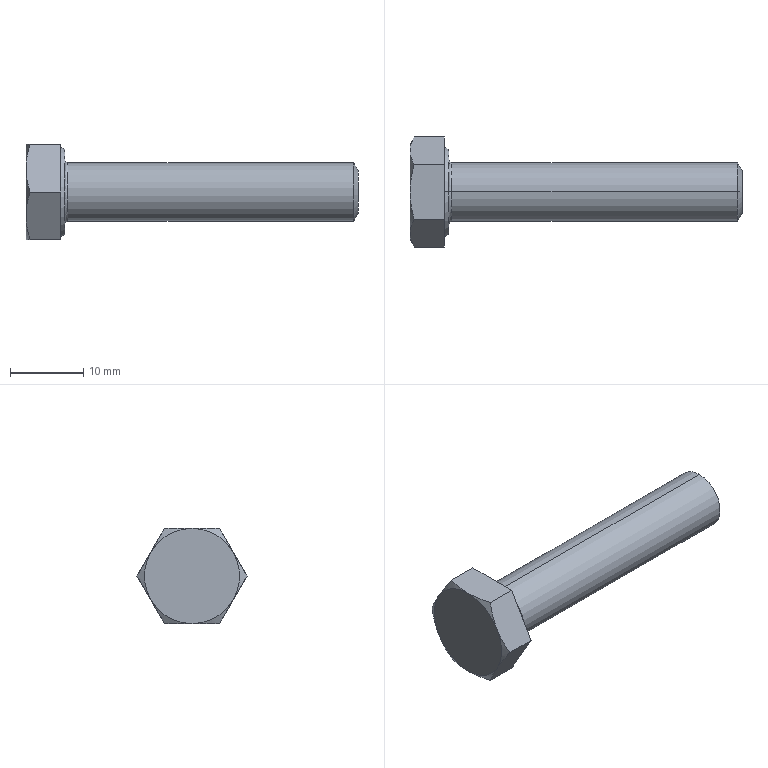Part | SolidWorks | features BaseBody 1, RefAxis 1 | 1 solid | 24 faces | box 45.3 x 15.011 x 13 mm | volume 2757 mm3 | cone 10 | plane 10 | spline 2 | cylinder 2 | commonest cylinder face diameters 8 x2
STEP:
#1=CARTESIAN_POINT('',(5.3,0.,4.4));
#2=VERTEX_POINT('',#1);
#3=CARTESIAN_POINT('',(5.3,0.,-4.4));
#4=VERTEX_POINT('',#3);
#5=CARTESIAN_POINT('',(5.3,0.,4.4));
#6=CARTESIAN_POINT('',(5.3,0.2797,4.4));
#7=CARTESIAN_POINT('',(5.3,0.6919,4.361));
#8=CARTESIAN_POINT('',(5.3,1.16,4.249));
#9=CARTESIAN_POINT('',(5.3,1.391,4.176));
#10=CARTESIAN_POINT('',(5.3,1.489,4.141));
#11=CARTESIAN_POINT('',(5.3,1.554,4.116));
#12=CARTESIAN_POINT('',(5.3,1.585,4.105));
#13=CARTESIAN_POINT('',(5.3,1.758,4.036));
#14=CARTESIAN_POINT('',(5.3,1.96,3.944));
#15=CARTESIAN_POINT('',(5.3,2.154,3.837));
#16=CARTESIAN_POINT('',(5.3,2.282,3.763));
#17=CARTESIAN_POINT('',(5.3,2.344,3.724));
#18=CARTESIAN_POINT('',(5.3,2.662,3.517));
#19=CARTESIAN_POINT('',(5.3,2.897,3.326));
#20=CARTESIAN_POINT('',(5.3,3.219,3.004));
#21=CARTESIAN_POINT('',(5.3,3.37,2.836));
#22=CARTESIAN_POINT('',(5.3,3.509,2.656));
#23=CARTESIAN_POINT('',(5.3,3.598,2.534));
#24=CARTESIAN_POINT('',(5.3,3.642,2.47));
#25=CARTESIAN_POINT('',(5.3,3.764,2.283));
#26=CARTESIAN_POINT('',(5.3,3.876,2.092));
#27=CARTESIAN_POINT('',(5.3,3.989,1.859));
#28=CARTESIAN_POINT('',(5.3,4.042,1.74));
#29=CARTESIAN_POINT('',(5.3,4.063,1.689));
#30=CARTESIAN_POINT('',(5.3,4.077,1.654));
#31=CARTESIAN_POINT('',(5.3,4.085,1.636));
#32=CARTESIAN_POINT('',(5.3,4.297,1.1));
#33=CARTESIAN_POINT('',(5.3,4.4,0.5592));
#34=CARTESIAN_POINT('',(5.3,4.4,-0.2796));
#35=CARTESIAN_POINT('',(5.3,4.361,-0.6917));
#36=CARTESIAN_POINT('',(5.3,4.249,-1.16));
#37=CARTESIAN_POINT('',(5.3,4.176,-1.391));
#38=CARTESIAN_POINT('',(5.3,4.141,-1.489));
#39=CARTESIAN_POINT('',(5.3,4.116,-1.554));
#40=CARTESIAN_POINT('',(5.3,4.105,-1.585));
#41=CARTESIAN_POINT('',(5.3,4.036,-1.758));
#42=CARTESIAN_POINT('',(5.3,3.944,-1.96));
#43=CARTESIAN_POINT('',(5.3,3.837,-2.154));
#44=CARTESIAN_POINT('',(5.3,3.763,-2.282));
#45=CARTESIAN_POINT('',(5.3,3.724,-2.344));
#46=CARTESIAN_POINT('',(5.3,3.517,-2.662));
#47=CARTESIAN_POINT('',(5.3,3.326,-2.897));
#48=CARTESIAN_POINT('',(5.3,3.004,-3.219));
#49=CARTESIAN_POINT('',(5.3,2.836,-3.37));
#50=CARTESIAN_POINT('',(5.3,2.656,-3.509));
#51=CARTESIAN_POINT('',(5.3,2.534,-3.598));
#52=CARTESIAN_POINT('',(5.3,2.47,-3.642));
#53=CARTESIAN_POINT('',(5.3,2.283,-3.764));
#54=CARTESIAN_POINT('',(5.3,2.092,-3.876));
#55=CARTESIAN_POINT('',(5.3,1.859,-3.989));
#56=CARTESIAN_POINT('',(5.3,1.74,-4.042));
#57=CARTESIAN_POINT('',(5.3,1.689,-4.063));
#58=CARTESIAN_POINT('',(5.3,1.654,-4.077));
#59=CARTESIAN_POINT('',(5.3,1.636,-4.085));
#60=CARTESIAN_POINT('',(5.3,1.1,-4.297));
#61=CARTESIAN_POINT('',(5.3,0.5597,-4.4));
#62=CARTESIAN_POINT('',(5.3,0.,-4.4));
#63=B_SPLINE_CURVE_WITH_KNOTS('',3,(#5,#6,#7,#8,#9,#10,#11,#12,#13,#14,#15,#16,#17,#18,#19,#20,#21,#22,#23,#24,#25,#26,#27,#28,#29,#30,#31,#32,#33,#34,#35,#36,#37,#38,#39,#40,#41,#42,#43,#44,#45,#46,#47,#48,#49,#50,#51,#52,#53,#54,#55,#56,#57,#58,#59,#60,#61,#62),.UNSPECIFIED.,.F.,.F.,(4,1,1,1,2,2,1,2,2,2,1,2,2,1,1,1,2,2,2,1,1,1,2,2,1,2,2,2,1,2,2,1,1,1,2,2,4),(0.,0.0625,0.09375,0.1094,0.1172,0.125,0.1562,0.1719,0.1875,0.25,0.2812,0.2969,0.3125,0.3437,0.3594,0.3672,0.3711,0.375,0.5,0.5625,0.5937,0.6094,0.6172,0.625,0.6562,0.6719,0.6875,0.75,0.7812,0.7969,0.8125,0.8437,0.8594,0.8672,0.8711,0.875,1.),.UNSPECIFIED.);
#64=EDGE_CURVE('',#2,#4,#63,.T.);
#65=ORIENTED_EDGE('',*,*,#64,.F.);
#66=CARTESIAN_POINT('',(5.7,0.,4.));
#67=VERTEX_POINT('',#66);
#68=CARTESIAN_POINT('',(5.7,0.,4.4));
#69=DIRECTION('',(0.,-1.,0.));
#70=DIRECTION('',(0.,0.,1.));
#71=AXIS2_PLACEMENT_3D('',#68,#69,#70);
#72=CIRCLE('',#71,0.4);
#73=EDGE_CURVE('',#2,#67,#72,.T.);
#74=ORIENTED_EDGE('',*,*,#73,.T.);
#75=CARTESIAN_POINT('',(5.7,0.,-4.));
#76=VERTEX_POINT('',#75);
#77=CARTESIAN_POINT('',(5.7,0.,0.));
#78=DIRECTION('',(1.,0.,0.));
#79=DIRECTION('',(0.,0.,1.));
#80=AXIS2_PLACEMENT_3D('',#77,#78,#79);
#81=CIRCLE('',#80,4.);
#82=EDGE_CURVE('',#76,#67,#81,.T.);
#83=ORIENTED_EDGE('',*,*,#82,.F.);
#84=CARTESIAN_POINT('',(5.7,0.,-4.4));
#85=DIRECTION('',(0.,1.,0.));
#86=DIRECTION('',(0.,0.,-1.));
#87=AXIS2_PLACEMENT_3D('',#84,#85,#86);
#88=CIRCLE('',#87,0.4);
#89=EDGE_CURVE('',#4,#76,#88,.T.);
#90=ORIENTED_EDGE('',*,*,#89,.F.);
#91=EDGE_LOOP('',(#65,#74,#83,#90));
#92=FACE_OUTER_BOUND('',#91,.T.);
#93=CARTESIAN_POINT('',(5.3,0.,-4.4));
#94=CARTESIAN_POINT('',(5.3,8.8,-4.4));
#95=CARTESIAN_POINT('',(5.3,8.8,4.4));
#96=CARTESIAN_POINT('',(5.3,0.,4.4));
#97=CARTESIAN_POINT('',(5.3,0.,-4.166));
#98=CARTESIAN_POINT('',(5.3,8.331,-4.166));
#99=CARTESIAN_POINT('',(5.3,8.331,4.166));
#100=CARTESIAN_POINT('',(5.3,0.,4.166));
#101=CARTESIAN_POINT('',(5.466,0.,-4.));
#102=CARTESIAN_POINT('',(5.466,8.,-4.));
#103=CARTESIAN_POINT('',(5.466,8.,4.));
#104=CARTESIAN_POINT('',(5.466,0.,4.));
#105=CARTESIAN_POINT('',(5.7,0.,-4.));
#106=CARTESIAN_POINT('',(5.7,8.,-4.));
#107=CARTESIAN_POINT('',(5.7,8.,4.));
#108=CARTESIAN_POINT('',(5.7,0.,4.));
#109=(BOUNDED_SURFACE()B_SPLINE_SURFACE(3,3,((#93,#94,#95,#96),(#97,#98,#99,#100),(#101,#102,#103,#104),(#105,#106,#107,#108)),.UNSPECIFIED.,.F.,.F.,.T.)B_SPLINE_SURFACE_WITH_KNOTS((4,4),(4,4),(0.,1.),(0.,1.),.UNSPECIFIED.)GEOMETRIC_REPRESENTATION_ITEM()RATIONAL_B_SPLINE_SURFACE(((1.,0.3333,0.3333,1.),(0.8047,0.2682,0.2682,0.8047),(0.8047,0.2682,0.2682,0.8047),(1.,0.3333,0.3333,1.)))REPRESENTATION_ITEM('')SURFACE());
#110=ADVANCED_FACE('',(#92),#109,.F.);
#111=CARTESIAN_POINT('',(44.675,0.,4.));
#112=VERTEX_POINT('',#111);
#113=CARTESIAN_POINT('',(44.675,0.,-4.));
#114=VERTEX_POINT('',#113);
#115=CARTESIAN_POINT('',(44.675,0.,0.));
#116=DIRECTION('',(-1.,0.,0.));
#117=DIRECTION('',(0.,0.,1.));
#118=AXIS2_PLACEMENT_3D('',#115,#116,#117);
#119=CIRCLE('',#118,4.);
#120=EDGE_CURVE('',#112,#114,#119,.T.);
#121=ORIENTED_EDGE('',*,*,#120,.T.);
#122=CARTESIAN_POINT('',(0.,0.,-4.));
#123=DIRECTION('',(-1.,0.,0.));
#124=VECTOR('',#123,1000.);
#125=LINE('',#122,#124);
#126=EDGE_CURVE('',#114,#76,#125,.T.);
#127=ORIENTED_EDGE('',*,*,#126,.T.);
#128=ORIENTED_EDGE('',*,*,#82,.T.);
#129=CARTESIAN_POINT('',(0.,0.,4.));
#130=DIRECTION('',(-1.,0.,0.));
#131=VECTOR('',#130,1000.);
#132=LINE('',#129,#131);
#133=EDGE_CURVE('',#112,#67,#132,.T.);
#134=ORIENTED_EDGE('',*,*,#133,.F.);
#135=EDGE_LOOP('',(#121,#127,#128,#134));
#136=FACE_OUTER_BOUND('',#135,.T.);
#137=CARTESIAN_POINT('',(0.,0.,0.));
#138=DIRECTION('',(-1.,0.,0.));
#139=DIRECTION('',(0.,0.,1.));
#140=AXIS2_PLACEMENT_3D('',#137,#138,#139);
#141=CYLINDRICAL_SURFACE('',#140,4.);
#142=ADVANCED_FACE('',(#136),#141,.T.);
#143=CARTESIAN_POINT('',(45.3,0.,2.917));
#144=VERTEX_POINT('',#143);
#145=CARTESIAN_POINT('',(45.3,0.,-2.917));
#146=VERTEX_POINT('',#145);
#147=CARTESIAN_POINT('',(45.3,0.,0.));
#148=DIRECTION('',(-1.,0.,0.));
#149=DIRECTION('',(0.,0.,1.));
#150=AXIS2_PLACEMENT_3D('',#147,#148,#149);
#151=CIRCLE('',#150,2.917);
#152=EDGE_CURVE('',#144,#146,#151,.T.);
#153=ORIENTED_EDGE('',*,*,#152,.T.);
#154=CARTESIAN_POINT('',(44.675,0.,-4.));
#155=DIRECTION('',(-0.5,0.,-0.866));
#156=VECTOR('',#155,1000.);
#157=LINE('',#154,#156);
#158=EDGE_CURVE('',#146,#114,#157,.T.);
#159=ORIENTED_EDGE('',*,*,#158,.T.);
#160=ORIENTED_EDGE('',*,*,#120,.F.);
#161=CARTESIAN_POINT('',(44.675,0.,4.));
#162=DIRECTION('',(-0.5,0.,0.866));
#163=VECTOR('',#162,1000.);
#164=LINE('',#161,#163);
#165=EDGE_CURVE('',#144,#112,#164,.T.);
#166=ORIENTED_EDGE('',*,*,#165,.F.);
#167=EDGE_LOOP('',(#153,#159,#160,#166));
#168=FACE_OUTER_BOUND('',#167,.T.);
#169=CARTESIAN_POINT('',(44.675,0.,0.));
#170=DIRECTION('',(-1.,0.,0.));
#171=DIRECTION('',(0.,0.,1.));
#172=AXIS2_PLACEMENT_3D('',#169,#170,#171);
#173=CONICAL_SURFACE('',#172,4.,1.047);
#174=ADVANCED_FACE('',(#168),#173,.T.);
#175=CARTESIAN_POINT('',(5.3,0.,-5.815));
#176=VERTEX_POINT('',#175);
#177=CARTESIAN_POINT('',(5.3,0.,5.815));
#178=VERTEX_POINT('',#177);
#179=CARTESIAN_POINT('',(5.3,0.,0.));
#180=DIRECTION('',(1.,0.,0.));
#181=DIRECTION('',(0.,0.,1.));
#182=AXIS2_PLACEMENT_3D('',#179,#180,#181);
#183=CIRCLE('',#182,5.815);
#184=EDGE_CURVE('',#176,#178,#183,.T.);
#185=ORIENTED_EDGE('',*,*,#184,.F.);
#186=CARTESIAN_POINT('',(4.7,0.,-6.161));
#187=VERTEX_POINT('',#186);
#188=CARTESIAN_POINT('',(4.7,0.,-6.161));
#189=DIRECTION('',(-0.866,0.,-0.5));
#190=VECTOR('',#189,1000.);
#191=LINE('',#188,#190);
#192=EDGE_CURVE('',#176,#187,#191,.T.);
#193=ORIENTED_EDGE('',*,*,#192,.T.);
#194=CARTESIAN_POINT('',(4.7,0.,6.161));
#195=VERTEX_POINT('',#194);
#196=CARTESIAN_POINT('',(4.7,0.,0.));
#197=DIRECTION('',(1.,0.,0.));
#198=DIRECTION('',(0.,0.,1.));
#199=AXIS2_PLACEMENT_3D('',#196,#197,#198);
#200=CIRCLE('',#199,6.161);
#201=EDGE_CURVE('',#187,#195,#200,.T.);
#202=ORIENTED_EDGE('',*,*,#201,.T.);
#203=CARTESIAN_POINT('',(4.7,0.,6.161));
#204=DIRECTION('',(-0.866,0.,0.5));
#205=VECTOR('',#204,1000.);
#206=LINE('',#203,#205);
#207=EDGE_CURVE('',#178,#195,#206,.T.);
#208=ORIENTED_EDGE('',*,*,#207,.F.);
#209=EDGE_LOOP('',(#185,#193,#202,#208));
#210=FACE_OUTER_BOUND('',#209,.T.);
#211=CARTESIAN_POINT('',(4.7,0.,0.));
#212=DIRECTION('',(-1.,0.,0.));
#213=DIRECTION('',(0.,0.,1.));
#214=AXIS2_PLACEMENT_3D('',#211,#212,#213);
#215=CONICAL_SURFACE('',#214,6.161,0.5236);
#216=ADVANCED_FACE('',(#210),#215,.T.);
#217=ORIENTED_EDGE('',*,*,#126,.F.);
#218=CARTESIAN_POINT('',(44.675,0.,0.));
#219=DIRECTION('',(-1.,0.,0.));
#220=DIRECTION('',(0.,0.,1.));
#221=AXIS2_PLACEMENT_3D('',#218,#219,#220);
#222=CIRCLE('',#221,4.);
#223=EDGE_CURVE('',#114,#112,#222,.T.);
#224=ORIENTED_EDGE('',*,*,#223,.T.);
#225=ORIENTED_EDGE('',*,*,#133,.T.);
#226=CARTESIAN_POINT('',(5.7,0.,0.));
#227=DIRECTION('',(1.,0.,0.));
#228=DIRECTION('',(0.,0.,1.));
#229=AXIS2_PLACEMENT_3D('',#226,#227,#228);
#230=CIRCLE('',#229,4.);
#231=EDGE_CURVE('',#67,#76,#230,.T.);
#232=ORIENTED_EDGE('',*,*,#231,.T.);
#233=EDGE_LOOP('',(#217,#224,#225,#232));
#234=FACE_OUTER_BOUND('',#233,.T.);
#235=CARTESIAN_POINT('',(0.,0.,0.));
#236=DIRECTION('',(-1.,0.,0.));
#237=DIRECTION('',(0.,0.,1.));
#238=AXIS2_PLACEMENT_3D('',#235,#236,#237);
#239=CYLINDRICAL_SURFACE('',#238,4.);
#240=ADVANCED_FACE('',(#234),#239,.T.);
#241=ORIENTED_EDGE('',*,*,#73,.F.);
#242=CARTESIAN_POINT('',(5.3,0.,-4.4));
#243=CARTESIAN_POINT('',(5.3,-0.2797,-4.4));
#244=CARTESIAN_POINT('',(5.3,-0.6919,-4.361));
#245=CARTESIAN_POINT('',(5.3,-1.16,-4.249));
#246=CARTESIAN_POINT('',(5.3,-1.391,-4.176));
#247=CARTESIAN_POINT('',(5.3,-1.489,-4.141));
#248=CARTESIAN_POINT('',(5.3,-1.554,-4.116));
#249=CARTESIAN_POINT('',(5.3,-1.585,-4.105));
#250=CARTESIAN_POINT('',(5.3,-1.758,-4.036));
#251=CARTESIAN_POINT('',(5.3,-1.96,-3.944));
#252=CARTESIAN_POINT('',(5.3,-2.154,-3.837));
#253=CARTESIAN_POINT('',(5.3,-2.282,-3.763));
#254=CARTESIAN_POINT('',(5.3,-2.344,-3.724));
#255=CARTESIAN_POINT('',(5.3,-2.662,-3.517));
#256=CARTESIAN_POINT('',(5.3,-2.897,-3.326));
#257=CARTESIAN_POINT('',(5.3,-3.219,-3.004));
#258=CARTESIAN_POINT('',(5.3,-3.37,-2.836));
#259=CARTESIAN_POINT('',(5.3,-3.509,-2.656));
#260=CARTESIAN_POINT('',(5.3,-3.598,-2.534));
#261=CARTESIAN_POINT('',(5.3,-3.642,-2.47));
#262=CARTESIAN_POINT('',(5.3,-3.764,-2.283));
#263=CARTESIAN_POINT('',(5.3,-3.876,-2.092));
#264=CARTESIAN_POINT('',(5.3,-3.989,-1.859));
#265=CARTESIAN_POINT('',(5.3,-4.042,-1.74));
#266=CARTESIAN_POINT('',(5.3,-4.063,-1.689));
#267=CARTESIAN_POINT('',(5.3,-4.077,-1.654));
#268=CARTESIAN_POINT('',(5.3,-4.085,-1.636));
#269=CARTESIAN_POINT('',(5.3,-4.297,-1.1));
#270=CARTESIAN_POINT('',(5.3,-4.4,-0.5592));
#271=CARTESIAN_POINT('',(5.3,-4.4,0.2796));
#272=CARTESIAN_POINT('',(5.3,-4.361,0.6917));
#273=CARTESIAN_POINT('',(5.3,-4.249,1.16));
#274=CARTESIAN_POINT('',(5.3,-4.176,1.391));
#275=CARTESIAN_POINT('',(5.3,-4.141,1.489));
#276=CARTESIAN_POINT('',(5.3,-4.116,1.554));
#277=CARTESIAN_POINT('',(5.3,-4.105,1.585));
#278=CARTESIAN_POINT('',(5.3,-4.036,1.758));
#279=CARTESIAN_POINT('',(5.3,-3.944,1.96));
#280=CARTESIAN_POINT('',(5.3,-3.837,2.154));
#281=CARTESIAN_POINT('',(5.3,-3.763,2.282));
#282=CARTESIAN_POINT('',(5.3,-3.724,2.344));
#283=CARTESIAN_POINT('',(5.3,-3.517,2.662));
#284=CARTESIAN_POINT('',(5.3,-3.326,2.897));
#285=CARTESIAN_POINT('',(5.3,-3.004,3.219));
#286=CARTESIAN_POINT('',(5.3,-2.836,3.37));
#287=CARTESIAN_POINT('',(5.3,-2.656,3.509));
#288=CARTESIAN_POINT('',(5.3,-2.534,3.598));
#289=CARTESIAN_POINT('',(5.3,-2.47,3.642));
#290=CARTESIAN_POINT('',(5.3,-2.283,3.764));
#291=CARTESIAN_POINT('',(5.3,-2.092,3.876));
#292=CARTESIAN_POINT('',(5.3,-1.859,3.989));
#293=CARTESIAN_POINT('',(5.3,-1.74,4.042));
#294=CARTESIAN_POINT('',(5.3,-1.689,4.063));
#295=CARTESIAN_POINT('',(5.3,-1.654,4.077));
#296=CARTESIAN_POINT('',(5.3,-1.636,4.085));
#297=CARTESIAN_POINT('',(5.3,-1.1,4.297));
#298=CARTESIAN_POINT('',(5.3,-0.5597,4.4));
#299=CARTESIAN_POINT('',(5.3,0.,4.4));
#300=B_SPLINE_CURVE_WITH_KNOTS('',3,(#242,#243,#244,#245,#246,#247,#248,#249,#250,#251,#252,#253,#254,#255,#256,#257,#258,#259,#260,#261,#262,#263,#264,#265,#266,#267,#268,#269,#270,#271,#272,#273,#274,#275,#276,#277,#278,#279,#280,#281,#282,#283,#284,#285,#286,#287,#288,#289,#290,#291,#292,#293,#294,#295,#296,#297,#298,#299),.UNSPECIFIED.,.F.,.F.,(4,1,1,1,2,2,1,2,2,2,1,2,2,1,1,1,2,2,2,1,1,1,2,2,1,2,2,2,1,2,2,1,1,1,2,2,4),(0.,0.0625,0.09375,0.1094,0.1172,0.125,0.1563,0.1719,0.1875,0.25,0.2813,0.2969,0.3125,0.3438,0.3594,0.3672,0.3711,0.375,0.5,0.5625,0.5938,0.6094,0.6172,0.625,0.6563,0.6719,0.6875,0.75,0.7813,0.7969,0.8125,0.8438,0.8594,0.8672,0.8711,0.875,1.),.UNSPECIFIED.);
#301=EDGE_CURVE('',#4,#2,#300,.T.);
#302=ORIENTED_EDGE('',*,*,#301,.F.);
#303=ORIENTED_EDGE('',*,*,#89,.T.);
#304=ORIENTED_EDGE('',*,*,#231,.F.);
#305=EDGE_LOOP('',(#241,#302,#303,#304));
#306=FACE_OUTER_BOUND('',#305,.T.);
#307=CARTESIAN_POINT('',(5.3,0.,4.4));
#308=CARTESIAN_POINT('',(5.3,-8.8,4.4));
#309=CARTESIAN_POINT('',(5.3,-8.8,-4.4));
#310=CARTESIAN_POINT('',(5.3,0.,-4.4));
#311=CARTESIAN_POINT('',(5.3,0.,4.166));
#312=CARTESIAN_POINT('',(5.3,-8.331,4.166));
#313=CARTESIAN_POINT('',(5.3,-8.331,-4.166));
#314=CARTESIAN_POINT('',(5.3,0.,-4.166));
#315=CARTESIAN_POINT('',(5.466,0.,4.));
#316=CARTESIAN_POINT('',(5.466,-8.,4.));
#317=CARTESIAN_POINT('',(5.466,-8.,-4.));
#318=CARTESIAN_POINT('',(5.466,0.,-4.));
#319=CARTESIAN_POINT('',(5.7,0.,4.));
#320=CARTESIAN_POINT('',(5.7,-8.,4.));
#321=CARTESIAN_POINT('',(5.7,-8.,-4.));
#322=CARTESIAN_POINT('',(5.7,0.,-4.));
#323=(BOUNDED_SURFACE()B_SPLINE_SURFACE(3,3,((#307,#308,#309,#310),(#311,#312,#313,#314),(#315,#316,#317,#318),(#319,#320,#321,#322)),.UNSPECIFIED.,.F.,.F.,.T.)B_SPLINE_SURFACE_WITH_KNOTS((4,4),(4,4),(0.,1.),(0.,1.),.UNSPECIFIED.)GEOMETRIC_REPRESENTATION_ITEM()RATIONAL_B_SPLINE_SURFACE(((1.,0.3333,0.3333,1.),(0.8047,0.2682,0.2682,0.8047),(0.8047,0.2682,0.2682,0.8047),(1.,0.3333,0.3333,1.)))REPRESENTATION_ITEM('')SURFACE());
#324=ADVANCED_FACE('',(#306),#323,.F.);
#325=ORIENTED_EDGE('',*,*,#158,.F.);
#326=CARTESIAN_POINT('',(45.3,0.,0.));
#327=DIRECTION('',(-1.,0.,0.));
#328=DIRECTION('',(0.,0.,1.));
#329=AXIS2_PLACEMENT_3D('',#326,#327,#328);
#330=CIRCLE('',#329,2.917);
#331=EDGE_CURVE('',#146,#144,#330,.T.);
#332=ORIENTED_EDGE('',*,*,#331,.T.);
#333=ORIENTED_EDGE('',*,*,#165,.T.);
#334=ORIENTED_EDGE('',*,*,#223,.F.);
#335=EDGE_LOOP('',(#325,#332,#333,#334));
#336=FACE_OUTER_BOUND('',#335,.T.);
#337=CARTESIAN_POINT('',(44.675,0.,0.));
#338=DIRECTION('',(-1.,0.,0.));
#339=DIRECTION('',(0.,0.,1.));
#340=AXIS2_PLACEMENT_3D('',#337,#338,#339);
#341=CONICAL_SURFACE('',#340,4.,1.047);
#342=ADVANCED_FACE('',(#336),#341,.T.);
#343=CARTESIAN_POINT('',(5.3,0.,0.));
#344=DIRECTION('',(1.,0.,0.));
#345=DIRECTION('',(0.,0.,1.));
#346=AXIS2_PLACEMENT_3D('',#343,#344,#345);
#347=CIRCLE('',#346,5.815);
#348=EDGE_CURVE('',#178,#176,#347,.T.);
#349=ORIENTED_EDGE('',*,*,#348,.T.);
#350=ORIENTED_EDGE('',*,*,#184,.T.);
#351=EDGE_LOOP('',(#349,#350));
#352=FACE_OUTER_BOUND('',#351,.T.);
#353=ORIENTED_EDGE('',*,*,#301,.T.);
#354=ORIENTED_EDGE('',*,*,#64,.T.);
#355=EDGE_LOOP('',(#353,#354));
#356=FACE_BOUND('',#355,.T.);
#357=CARTESIAN_POINT('',(5.3,0.,-13.));
#358=DIRECTION('',(1.,0.,0.));
#359=DIRECTION('',(0.,0.,-1.));
#360=AXIS2_PLACEMENT_3D('',#357,#358,#359);
#361=PLANE('',#360);
#362=ADVANCED_FACE('',(#352,#356),#361,.T.);
#363=ORIENTED_EDGE('',*,*,#152,.F.);
#364=ORIENTED_EDGE('',*,*,#331,.F.);
#365=EDGE_LOOP('',(#363,#364));
#366=FACE_OUTER_BOUND('',#365,.T.);
#367=CARTESIAN_POINT('',(45.3,0.,0.));
#368=DIRECTION('',(-1.,0.,0.));
#369=DIRECTION('',(0.,0.,1.));
#370=AXIS2_PLACEMENT_3D('',#367,#368,#369);
#371=PLANE('',#370);
#372=ADVANCED_FACE('',(#366),#371,.F.);
#373=ORIENTED_EDGE('',*,*,#192,.F.);
#374=ORIENTED_EDGE('',*,*,#348,.F.);
#375=ORIENTED_EDGE('',*,*,#207,.T.);
#376=CARTESIAN_POINT('',(4.7,0.,0.));
#377=DIRECTION('',(1.,0.,0.));
#378=DIRECTION('',(0.,0.,1.));
#379=AXIS2_PLACEMENT_3D('',#376,#377,#378);
#380=CIRCLE('',#379,6.161);
#381=EDGE_CURVE('',#195,#187,#380,.T.);
#382=ORIENTED_EDGE('',*,*,#381,.T.);
#383=EDGE_LOOP('',(#373,#374,#375,#382));
#384=FACE_OUTER_BOUND('',#383,.T.);
#385=CARTESIAN_POINT('',(4.7,0.,0.));
#386=DIRECTION('',(-1.,0.,0.));
#387=DIRECTION('',(0.,0.,1.));
#388=AXIS2_PLACEMENT_3D('',#385,#386,#387);
#389=CONICAL_SURFACE('',#388,6.161,0.5236);
#390=ADVANCED_FACE('',(#384),#389,.T.);
#391=CARTESIAN_POINT('',(4.7,-7.506,0.));
#392=VERTEX_POINT('',#391);
#393=CARTESIAN_POINT('',(4.7,-3.753,-6.5));
#394=VERTEX_POINT('',#393);
#395=CARTESIAN_POINT('',(4.7,-7.506,0.));
#396=DIRECTION('',(0.,0.5,-0.866));
#397=VECTOR('',#396,1000.);
#398=LINE('',#395,#397);
#399=EDGE_CURVE('',#392,#394,#398,.T.);
#400=ORIENTED_EDGE('',*,*,#399,.T.);
#401=CARTESIAN_POINT('',(4.7,3.753,-6.5));
#402=VERTEX_POINT('',#401);
#403=CARTESIAN_POINT('',(4.7,6.161,-6.5));
#404=DIRECTION('',(0.,1.,0.));
#405=VECTOR('',#404,1000.);
#406=LINE('',#403,#405);
#407=EDGE_CURVE('',#394,#402,#406,.T.);
#408=ORIENTED_EDGE('',*,*,#407,.T.);
#409=CARTESIAN_POINT('',(4.7,7.506,0.));
#410=VERTEX_POINT('',#409);
#411=CARTESIAN_POINT('',(4.7,3.753,-6.5));
#412=DIRECTION('',(0.,0.5,0.866));
#413=VECTOR('',#412,1000.);
#414=LINE('',#411,#413);
#415=EDGE_CURVE('',#402,#410,#414,.T.);
#416=ORIENTED_EDGE('',*,*,#415,.T.);
#417=CARTESIAN_POINT('',(4.7,3.753,6.5));
#418=VERTEX_POINT('',#417);
#419=CARTESIAN_POINT('',(4.7,7.506,0.));
#420=DIRECTION('',(0.,-0.5,0.866));
#421=VECTOR('',#420,1000.);
#422=LINE('',#419,#421);
#423=EDGE_CURVE('',#410,#418,#422,.T.);
#424=ORIENTED_EDGE('',*,*,#423,.T.);
#425=CARTESIAN_POINT('',(4.7,-3.753,6.5));
#426=VERTEX_POINT('',#425);
#427=CARTESIAN_POINT('',(4.7,6.161,6.5));
#428=DIRECTION('',(0.,-1.,0.));
#429=VECTOR('',#428,1000.);
#430=LINE('',#427,#429);
#431=EDGE_CURVE('',#418,#426,#430,.T.);
#432=ORIENTED_EDGE('',*,*,#431,.T.);
#433=CARTESIAN_POINT('',(4.7,-3.753,6.5));
#434=DIRECTION('',(0.,-0.5,-0.866));
#435=VECTOR('',#434,1000.);
#436=LINE('',#433,#435);
#437=EDGE_CURVE('',#426,#392,#436,.T.);
#438=ORIENTED_EDGE('',*,*,#437,.T.);
#439=EDGE_LOOP('',(#400,#408,#416,#424,#432,#438));
#440=FACE_OUTER_BOUND('',#439,.T.);
#441=ORIENTED_EDGE('',*,*,#381,.F.);
#442=ORIENTED_EDGE('',*,*,#201,.F.);
#443=EDGE_LOOP('',(#441,#442));
#444=FACE_BOUND('',#443,.T.);
#445=CARTESIAN_POINT('',(4.7,6.161,0.));
#446=DIRECTION('',(1.,0.,0.));
#447=DIRECTION('',(0.,0.,-1.));
#448=AXIS2_PLACEMENT_3D('',#445,#446,#447);
#449=PLANE('',#448);
#450=ADVANCED_FACE('',(#440,#444),#449,.T.);
#451=CARTESIAN_POINT('',(0.5806,-3.753,-6.5));
#452=VERTEX_POINT('',#451);
#453=CARTESIAN_POINT('',(5.3,-3.753,-6.5));
#454=DIRECTION('',(1.,0.,0.));
#455=VECTOR('',#454,1000.);
#456=LINE('',#453,#455);
#457=EDGE_CURVE('',#452,#394,#456,.T.);
#458=ORIENTED_EDGE('',*,*,#457,.F.);
#459=CARTESIAN_POINT('',(0.,0.,-6.5));
#460=VERTEX_POINT('',#459);
#461=CARTESIAN_POINT('',(0.,0.,-6.5));
#462=CARTESIAN_POINT('',(0.,-1.281,-6.5));
#463=CARTESIAN_POINT('',(0.2266,-2.527,-6.5));
#464=CARTESIAN_POINT('',(0.5806,-3.753,-6.5));
#465=B_SPLINE_CURVE_WITH_KNOTS('',3,(#461,#462,#463,#464),.UNSPECIFIED.,.F.,.F.,(4,4),(0.,0.003797),.UNSPECIFIED.);
#466=EDGE_CURVE('',#460,#452,#465,.T.);
#467=ORIENTED_EDGE('',*,*,#466,.F.);
#468=CARTESIAN_POINT('',(0.5806,3.753,-6.5));
#469=VERTEX_POINT('',#468);
#470=CARTESIAN_POINT('',(0.5806,3.753,-6.5));
#471=CARTESIAN_POINT('',(0.2266,2.527,-6.5));
#472=CARTESIAN_POINT('',(0.,1.281,-6.5));
#473=CARTESIAN_POINT('',(0.,0.,-6.5));
#474=B_SPLINE_CURVE_WITH_KNOTS('',3,(#470,#471,#472,#473),.UNSPECIFIED.,.F.,.F.,(4,4),(0.,0.003797),.UNSPECIFIED.);
#475=EDGE_CURVE('',#469,#460,#474,.T.);
#476=ORIENTED_EDGE('',*,*,#475,.F.);
#477=CARTESIAN_POINT('',(5.3,3.753,-6.5));
#478=DIRECTION('',(-1.,0.,0.));
#479=VECTOR('',#478,1000.);
#480=LINE('',#477,#479);
#481=EDGE_CURVE('',#402,#469,#480,.T.);
#482=ORIENTED_EDGE('',*,*,#481,.F.);
#483=ORIENTED_EDGE('',*,*,#407,.F.);
#484=EDGE_LOOP('',(#458,#467,#476,#482,#483));
#485=FACE_OUTER_BOUND('',#484,.T.);
#486=CARTESIAN_POINT('',(5.3,3.753,-6.5));
#487=DIRECTION('',(0.,0.,1.));
#488=DIRECTION('',(0.,-1.,0.));
#489=AXIS2_PLACEMENT_3D('',#486,#487,#488);
#490=PLANE('',#489);
#491=ADVANCED_FACE('',(#485),#490,.F.);
#492=CARTESIAN_POINT('',(0.5806,-7.506,0.));
#493=VERTEX_POINT('',#492);
#494=CARTESIAN_POINT('',(5.3,-7.506,0.));
#495=DIRECTION('',(1.,0.,0.));
#496=VECTOR('',#495,1000.);
#497=LINE('',#494,#496);
#498=EDGE_CURVE('',#493,#392,#497,.T.);
#499=ORIENTED_EDGE('',*,*,#498,.F.);
#500=CARTESIAN_POINT('',(0.,-5.629,-3.25));
#501=VERTEX_POINT('',#500);
#502=CARTESIAN_POINT('',(0.,-5.629,-3.25));
#503=CARTESIAN_POINT('',(0.,-6.27,-2.141));
#504=CARTESIAN_POINT('',(0.2266,-6.892,-1.062));
#505=CARTESIAN_POINT('',(0.5806,-7.506,0.));
#506=B_SPLINE_CURVE_WITH_KNOTS('',3,(#502,#503,#504,#505),.UNSPECIFIED.,.F.,.F.,(4,4),(0.,0.003797),.UNSPECIFIED.);
#507=EDGE_CURVE('',#501,#493,#506,.T.);
#508=ORIENTED_EDGE('',*,*,#507,.F.);
#509=CARTESIAN_POINT('',(0.5806,-3.753,-6.5));
#510=CARTESIAN_POINT('',(0.2266,-4.366,-5.438));
#511=CARTESIAN_POINT('',(0.,-4.989,-4.359));
#512=CARTESIAN_POINT('',(0.,-5.629,-3.25));
#513=B_SPLINE_CURVE_WITH_KNOTS('',3,(#509,#510,#511,#512),.UNSPECIFIED.,.F.,.F.,(4,4),(0.,0.003797),.UNSPECIFIED.);
#514=EDGE_CURVE('',#452,#501,#513,.T.);
#515=ORIENTED_EDGE('',*,*,#514,.F.);
#516=ORIENTED_EDGE('',*,*,#457,.T.);
#517=ORIENTED_EDGE('',*,*,#399,.F.);
#518=EDGE_LOOP('',(#499,#508,#515,#516,#517));
#519=FACE_OUTER_BOUND('',#518,.T.);
#520=CARTESIAN_POINT('',(5.3,-3.753,-6.5));
#521=DIRECTION('',(0.,0.866,0.5));
#522=DIRECTION('',(0.,-0.5,0.866));
#523=AXIS2_PLACEMENT_3D('',#520,#521,#522);
#524=PLANE('',#523);
#525=ADVANCED_FACE('',(#519),#524,.F.);
#526=CARTESIAN_POINT('',(0.5806,-3.753,6.5));
#527=VERTEX_POINT('',#526);
#528=CARTESIAN_POINT('',(5.3,-3.753,6.5));
#529=DIRECTION('',(1.,0.,0.));
#530=VECTOR('',#529,1000.);
#531=LINE('',#528,#530);
#532=EDGE_CURVE('',#527,#426,#531,.T.);
#533=ORIENTED_EDGE('',*,*,#532,.F.);
#534=CARTESIAN_POINT('',(0.,-5.629,3.25));
#535=VERTEX_POINT('',#534);
#536=CARTESIAN_POINT('',(0.,-5.629,3.25));
#537=CARTESIAN_POINT('',(0.,-4.989,4.359));
#538=CARTESIAN_POINT('',(0.2266,-4.366,5.438));
#539=CARTESIAN_POINT('',(0.5806,-3.753,6.5));
#540=B_SPLINE_CURVE_WITH_KNOTS('',3,(#536,#537,#538,#539),.UNSPECIFIED.,.F.,.F.,(4,4),(0.,0.003797),.UNSPECIFIED.);
#541=EDGE_CURVE('',#535,#527,#540,.T.);
#542=ORIENTED_EDGE('',*,*,#541,.F.);
#543=CARTESIAN_POINT('',(0.5806,-7.506,0.));
#544=CARTESIAN_POINT('',(0.2266,-6.892,1.062));
#545=CARTESIAN_POINT('',(0.,-6.27,2.141));
#546=CARTESIAN_POINT('',(0.,-5.629,3.25));
#547=B_SPLINE_CURVE_WITH_KNOTS('',3,(#543,#544,#545,#546),.UNSPECIFIED.,.F.,.F.,(4,4),(0.,0.003797),.UNSPECIFIED.);
#548=EDGE_CURVE('',#493,#535,#547,.T.);
#549=ORIENTED_EDGE('',*,*,#548,.F.);
#550=ORIENTED_EDGE('',*,*,#498,.T.);
#551=ORIENTED_EDGE('',*,*,#437,.F.);
#552=EDGE_LOOP('',(#533,#542,#549,#550,#551));
#553=FACE_OUTER_BOUND('',#552,.T.);
#554=CARTESIAN_POINT('',(5.3,-7.506,0.));
#555=DIRECTION('',(0.,0.866,-0.5));
#556=DIRECTION('',(0.,0.5,0.866));
#557=AXIS2_PLACEMENT_3D('',#554,#555,#556);
#558=PLANE('',#557);
#559=ADVANCED_FACE('',(#553),#558,.F.);
#560=CARTESIAN_POINT('',(0.5806,3.753,6.5));
#561=VERTEX_POINT('',#560);
#562=CARTESIAN_POINT('',(5.3,3.753,6.5));
#563=DIRECTION('',(1.,0.,0.));
#564=VECTOR('',#563,1000.);
#565=LINE('',#562,#564);
#566=EDGE_CURVE('',#561,#418,#565,.T.);
#567=ORIENTED_EDGE('',*,*,#566,.F.);
#568=CARTESIAN_POINT('',(0.,0.,6.5));
#569=VERTEX_POINT('',#568);
#570=CARTESIAN_POINT('',(0.,0.,6.5));
#571=CARTESIAN_POINT('',(0.,1.281,6.5));
#572=CARTESIAN_POINT('',(0.2266,2.527,6.5));
#573=CARTESIAN_POINT('',(0.5806,3.753,6.5));
#574=B_SPLINE_CURVE_WITH_KNOTS('',3,(#570,#571,#572,#573),.UNSPECIFIED.,.F.,.F.,(4,4),(0.,0.003797),.UNSPECIFIED.);
#575=EDGE_CURVE('',#569,#561,#574,.T.);
#576=ORIENTED_EDGE('',*,*,#575,.F.);
#577=CARTESIAN_POINT('',(0.5806,-3.753,6.5));
#578=CARTESIAN_POINT('',(0.2266,-2.527,6.5));
#579=CARTESIAN_POINT('',(0.,-1.281,6.5));
#580=CARTESIAN_POINT('',(0.,0.,6.5));
#581=B_SPLINE_CURVE_WITH_KNOTS('',3,(#577,#578,#579,#580),.UNSPECIFIED.,.F.,.F.,(4,4),(0.,0.003797),.UNSPECIFIED.);
#582=EDGE_CURVE('',#527,#569,#581,.T.);
#583=ORIENTED_EDGE('',*,*,#582,.F.);
#584=ORIENTED_EDGE('',*,*,#532,.T.);
#585=ORIENTED_EDGE('',*,*,#431,.F.);
#586=EDGE_LOOP('',(#567,#576,#583,#584,#585));
#587=FACE_OUTER_BOUND('',#586,.T.);
#588=CARTESIAN_POINT('',(5.3,3.753,6.5));
#589=DIRECTION('',(0.,0.,-1.));
#590=DIRECTION('',(-1.,0.,0.));
#591=AXIS2_PLACEMENT_3D('',#588,#589,#590);
#592=PLANE('',#591);
#593=ADVANCED_FACE('',(#587),#592,.F.);
#594=CARTESIAN_POINT('',(0.5806,7.506,0.));
#595=VERTEX_POINT('',#594);
#596=CARTESIAN_POINT('',(5.3,7.506,0.));
#597=DIRECTION('',(1.,0.,0.));
#598=VECTOR('',#597,1000.);
#599=LINE('',#596,#598);
#600=EDGE_CURVE('',#595,#410,#599,.T.);
#601=ORIENTED_EDGE('',*,*,#600,.F.);
#602=CARTESIAN_POINT('',(0.,5.629,3.25));
#603=VERTEX_POINT('',#602);
#604=CARTESIAN_POINT('',(0.,5.629,3.25));
#605=CARTESIAN_POINT('',(0.,6.27,2.141));
#606=CARTESIAN_POINT('',(0.2266,6.892,1.062));
#607=CARTESIAN_POINT('',(0.5806,7.506,0.));
#608=B_SPLINE_CURVE_WITH_KNOTS('',3,(#604,#605,#606,#607),.UNSPECIFIED.,.F.,.F.,(4,4),(0.,0.003797),.UNSPECIFIED.);
#609=EDGE_CURVE('',#603,#595,#608,.T.);
#610=ORIENTED_EDGE('',*,*,#609,.F.);
#611=CARTESIAN_POINT('',(0.5806,3.753,6.5));
#612=CARTESIAN_POINT('',(0.2266,4.366,5.438));
#613=CARTESIAN_POINT('',(0.,4.989,4.359));
#614=CARTESIAN_POINT('',(0.,5.629,3.25));
#615=B_SPLINE_CURVE_WITH_KNOTS('',3,(#611,#612,#613,#614),.UNSPECIFIED.,.F.,.F.,(4,4),(0.,0.003797),.UNSPECIFIED.);
#616=EDGE_CURVE('',#561,#603,#615,.T.);
#617=ORIENTED_EDGE('',*,*,#616,.F.);
#618=ORIENTED_EDGE('',*,*,#566,.T.);
#619=ORIENTED_EDGE('',*,*,#423,.F.);
#620=EDGE_LOOP('',(#601,#610,#617,#618,#619));
#621=FACE_OUTER_BOUND('',#620,.T.);
#622=CARTESIAN_POINT('',(5.3,7.506,0.));
#623=DIRECTION('',(0.,-0.866,-0.5));
#624=DIRECTION('',(0.,0.5,-0.866));
#625=AXIS2_PLACEMENT_3D('',#622,#623,#624);
#626=PLANE('',#625);
#627=ADVANCED_FACE('',(#621),#626,.F.);
#628=ORIENTED_EDGE('',*,*,#481,.T.);
#629=CARTESIAN_POINT('',(0.,5.629,-3.25));
#630=VERTEX_POINT('',#629);
#631=CARTESIAN_POINT('',(0.,5.629,-3.25));
#632=CARTESIAN_POINT('',(0.,4.989,-4.359));
#633=CARTESIAN_POINT('',(0.2266,4.366,-5.438));
#634=CARTESIAN_POINT('',(0.5806,3.753,-6.5));
#635=B_SPLINE_CURVE_WITH_KNOTS('',3,(#631,#632,#633,#634),.UNSPECIFIED.,.F.,.F.,(4,4),(0.,0.003797),.UNSPECIFIED.);
#636=EDGE_CURVE('',#630,#469,#635,.T.);
#637=ORIENTED_EDGE('',*,*,#636,.F.);
#638=CARTESIAN_POINT('',(0.5806,7.506,0.));
#639=CARTESIAN_POINT('',(0.2266,6.892,-1.062));
#640=CARTESIAN_POINT('',(0.,6.27,-2.141));
#641=CARTESIAN_POINT('',(0.,5.629,-3.25));
#642=B_SPLINE_CURVE_WITH_KNOTS('',3,(#638,#639,#640,#641),.UNSPECIFIED.,.F.,.F.,(4,4),(0.,0.003797),.UNSPECIFIED.);
#643=EDGE_CURVE('',#595,#630,#642,.T.);
#644=ORIENTED_EDGE('',*,*,#643,.F.);
#645=ORIENTED_EDGE('',*,*,#600,.T.);
#646=ORIENTED_EDGE('',*,*,#415,.F.);
#647=EDGE_LOOP('',(#628,#637,#644,#645,#646));
#648=FACE_OUTER_BOUND('',#647,.T.);
#649=CARTESIAN_POINT('',(5.3,3.753,-6.5));
#650=DIRECTION('',(0.,-0.866,0.5));
#651=DIRECTION('',(0.,-0.5,-0.866));
#652=AXIS2_PLACEMENT_3D('',#649,#650,#651);
#653=PLANE('',#652);
#654=ADVANCED_FACE('',(#648),#653,.F.);
#655=CARTESIAN_POINT('',(0.,0.,0.));
#656=DIRECTION('',(1.,0.,0.));
#657=DIRECTION('',(0.,0.,-1.));
#658=AXIS2_PLACEMENT_3D('',#655,#656,#657);
#659=CIRCLE('',#658,6.5);
#660=EDGE_CURVE('',#501,#460,#659,.T.);
#661=ORIENTED_EDGE('',*,*,#660,.T.);
#662=ORIENTED_EDGE('',*,*,#466,.T.);
#663=ORIENTED_EDGE('',*,*,#514,.T.);
#664=EDGE_LOOP('',(#661,#662,#663));
#665=FACE_OUTER_BOUND('',#664,.T.);
#666=CARTESIAN_POINT('',(0.584,0.,0.));
#667=DIRECTION('',(1.,0.,0.));
#668=DIRECTION('',(0.,0.,-1.));
#669=AXIS2_PLACEMENT_3D('',#666,#667,#668);
#670=CONICAL_SURFACE('',#669,7.512,1.047);
#671=ADVANCED_FACE('',(#665),#670,.T.);
#672=ORIENTED_EDGE('',*,*,#475,.T.);
#673=CARTESIAN_POINT('',(0.,0.,0.));
#674=DIRECTION('',(1.,0.,0.));
#675=DIRECTION('',(0.,0.,-1.));
#676=AXIS2_PLACEMENT_3D('',#673,#674,#675);
#677=CIRCLE('',#676,6.5);
#678=EDGE_CURVE('',#460,#630,#677,.T.);
#679=ORIENTED_EDGE('',*,*,#678,.T.);
#680=ORIENTED_EDGE('',*,*,#636,.T.);
#681=EDGE_LOOP('',(#672,#679,#680));
#682=FACE_OUTER_BOUND('',#681,.T.);
#683=CARTESIAN_POINT('',(0.584,0.,0.));
#684=DIRECTION('',(1.,0.,0.));
#685=DIRECTION('',(0.,0.,-1.));
#686=AXIS2_PLACEMENT_3D('',#683,#684,#685);
#687=CONICAL_SURFACE('',#686,7.512,1.047);
#688=ADVANCED_FACE('',(#682),#687,.T.);
#689=CARTESIAN_POINT('',(0.,0.,0.));
#690=DIRECTION('',(1.,0.,0.));
#691=DIRECTION('',(0.,0.,-1.));
#692=AXIS2_PLACEMENT_3D('',#689,#690,#691);
#693=CIRCLE('',#692,6.5);
#694=EDGE_CURVE('',#535,#501,#693,.T.);
#695=ORIENTED_EDGE('',*,*,#694,.T.);
#696=ORIENTED_EDGE('',*,*,#507,.T.);
#697=ORIENTED_EDGE('',*,*,#548,.T.);
#698=EDGE_LOOP('',(#695,#696,#697));
#699=FACE_OUTER_BOUND('',#698,.T.);
#700=CARTESIAN_POINT('',(0.584,0.,0.));
#701=DIRECTION('',(1.,0.,0.));
#702=DIRECTION('',(0.,0.,-1.));
#703=AXIS2_PLACEMENT_3D('',#700,#701,#702);
#704=CONICAL_SURFACE('',#703,7.512,1.047);
#705=ADVANCED_FACE('',(#699),#704,.T.);
#706=CARTESIAN_POINT('',(0.,0.,0.));
#707=DIRECTION('',(1.,0.,0.));
#708=DIRECTION('',(0.,0.,-1.));
#709=AXIS2_PLACEMENT_3D('',#706,#707,#708);
#710=CIRCLE('',#709,6.5);
#711=EDGE_CURVE('',#569,#535,#710,.T.);
#712=ORIENTED_EDGE('',*,*,#711,.T.);
#713=ORIENTED_EDGE('',*,*,#541,.T.);
#714=ORIENTED_EDGE('',*,*,#582,.T.);
#715=EDGE_LOOP('',(#712,#713,#714));
#716=FACE_OUTER_BOUND('',#715,.T.);
#717=CARTESIAN_POINT('',(0.584,0.,0.));
#718=DIRECTION('',(1.,0.,0.));
#719=DIRECTION('',(0.,0.,-1.));
#720=AXIS2_PLACEMENT_3D('',#717,#718,#719);
#721=CONICAL_SURFACE('',#720,7.512,1.047);
#722=ADVANCED_FACE('',(#716),#721,.T.);
#723=ORIENTED_EDGE('',*,*,#616,.T.);
#724=CARTESIAN_POINT('',(0.,0.,0.));
#725=DIRECTION('',(1.,0.,0.));
#726=DIRECTION('',(0.,0.,-1.));
#727=AXIS2_PLACEMENT_3D('',#724,#725,#726);
#728=CIRCLE('',#727,6.5);
#729=EDGE_CURVE('',#603,#569,#728,.T.);
#730=ORIENTED_EDGE('',*,*,#729,.T.);
#731=ORIENTED_EDGE('',*,*,#575,.T.);
#732=EDGE_LOOP('',(#723,#730,#731));
#733=FACE_OUTER_BOUND('',#732,.T.);
#734=CARTESIAN_POINT('',(0.584,0.,0.));
#735=DIRECTION('',(1.,0.,0.));
#736=DIRECTION('',(0.,0.,-1.));
#737=AXIS2_PLACEMENT_3D('',#734,#735,#736);
#738=CONICAL_SURFACE('',#737,7.512,1.047);
#739=ADVANCED_FACE('',(#733),#738,.T.);
#740=ORIENTED_EDGE('',*,*,#643,.T.);
#741=CARTESIAN_POINT('',(0.,0.,0.));
#742=DIRECTION('',(1.,0.,0.));
#743=DIRECTION('',(0.,0.,-1.));
#744=AXIS2_PLACEMENT_3D('',#741,#742,#743);
#745=CIRCLE('',#744,6.5);
#746=EDGE_CURVE('',#630,#603,#745,.T.);
#747=ORIENTED_EDGE('',*,*,#746,.T.);
#748=ORIENTED_EDGE('',*,*,#609,.T.);
#749=EDGE_LOOP('',(#740,#747,#748));
#750=FACE_OUTER_BOUND('',#749,.T.);
#751=CARTESIAN_POINT('',(0.584,0.,0.));
#752=DIRECTION('',(1.,0.,0.));
#753=DIRECTION('',(0.,0.,-1.));
#754=AXIS2_PLACEMENT_3D('',#751,#752,#753);
#755=CONICAL_SURFACE('',#754,7.512,1.047);
#756=ADVANCED_FACE('',(#750),#755,.T.);
#757=ORIENTED_EDGE('',*,*,#660,.F.);
#758=ORIENTED_EDGE('',*,*,#694,.F.);
#759=ORIENTED_EDGE('',*,*,#711,.F.);
#760=ORIENTED_EDGE('',*,*,#729,.F.);
#761=ORIENTED_EDGE('',*,*,#746,.F.);
#762=ORIENTED_EDGE('',*,*,#678,.F.);
#763=EDGE_LOOP('',(#757,#758,#759,#760,#761,#762));
#764=FACE_OUTER_BOUND('',#763,.T.);
#765=CARTESIAN_POINT('',(0.,0.,-13.));
#766=DIRECTION('',(1.,0.,0.));
#767=DIRECTION('',(0.,0.,-1.));
#768=AXIS2_PLACEMENT_3D('',#765,#766,#767);
#769=PLANE('',#768);
#770=ADVANCED_FACE('',(#764),#769,.F.);
#771=CLOSED_SHELL('',(#110,#142,#174,#216,#240,#324,#342,#362,#372,#390,#450,#491,#525,#559,#593,#627,#654,#671,#688,#705,#722,#739,#756,#770));
#772=MANIFOLD_SOLID_BREP('',#771);
#773=CARTESIAN_POINT('',(0.,0.,0.));
#774=DIRECTION('',(0.,0.,1.));
#775=DIRECTION('',(1.,0.,0.));
#776=AXIS2_PLACEMENT_3D('',#773,#774,#775);
#777=(LENGTH_UNIT()NAMED_UNIT(*)SI_UNIT(.MILLI.,.METRE.));
#778=UNCERTAINTY_MEASURE_WITH_UNIT(LENGTH_MEASURE(0.00001),#777,'','');
#779=(NAMED_UNIT(*)PLANE_ANGLE_UNIT()SI_UNIT($,.RADIAN.));
#780=(NAMED_UNIT(*)SI_UNIT($,.STERADIAN.)SOLID_ANGLE_UNIT());
#781=(GEOMETRIC_REPRESENTATION_CONTEXT(3)GLOBAL_UNCERTAINTY_ASSIGNED_CONTEXT((#778))GLOBAL_UNIT_ASSIGNED_CONTEXT((#777,#779,#780))REPRESENTATION_CONTEXT('',''));
#782=ADVANCED_BREP_SHAPE_REPRESENTATION('',(#772,#776),#781);